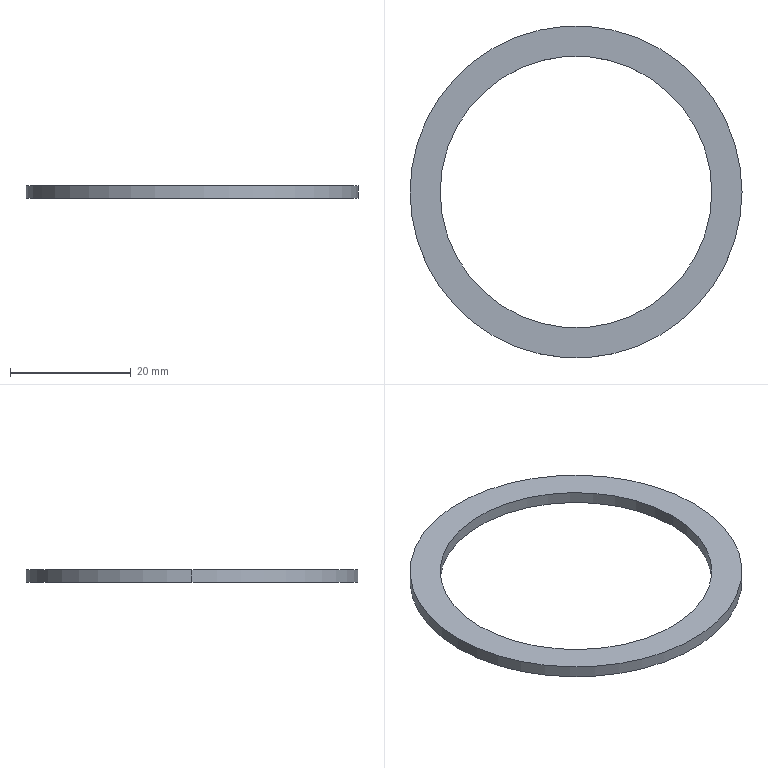Part | SolidWorks | features Extrusion 1 | 1 solid | 6 faces | box 55 x 55 x 2 mm | volume 1571 mm3 | cylinder 4 | plane 2 | commonest cylinder face diameters 45 x2 55 x2
STEP:
#1=CARTESIAN_POINT('',(-22.5,0.,2.));
#2=VERTEX_POINT('',#1);
#3=CARTESIAN_POINT('',(22.5,0.,2.));
#4=VERTEX_POINT('',#3);
#5=CARTESIAN_POINT('',(0.,0.,2.));
#6=DIRECTION('',(0.,0.,1.));
#7=DIRECTION('',(1.,0.,0.));
#8=AXIS2_PLACEMENT_3D('',#5,#6,#7);
#9=CIRCLE('',#8,22.5);
#10=EDGE_CURVE('',#2,#4,#9,.T.);
#11=ORIENTED_EDGE('',*,*,#10,.T.);
#12=CARTESIAN_POINT('',(22.5,0.,0.));
#13=VERTEX_POINT('',#12);
#14=CARTESIAN_POINT('',(22.5,0.,2.));
#15=DIRECTION('',(0.,0.,-1.));
#16=VECTOR('',#15,1000.);
#17=LINE('',#14,#16);
#18=EDGE_CURVE('',#4,#13,#17,.T.);
#19=ORIENTED_EDGE('',*,*,#18,.T.);
#20=CARTESIAN_POINT('',(-22.5,0.,0.));
#21=VERTEX_POINT('',#20);
#22=CARTESIAN_POINT('',(0.,0.,0.));
#23=DIRECTION('',(0.,0.,1.));
#24=DIRECTION('',(1.,0.,0.));
#25=AXIS2_PLACEMENT_3D('',#22,#23,#24);
#26=CIRCLE('',#25,22.5);
#27=EDGE_CURVE('',#21,#13,#26,.T.);
#28=ORIENTED_EDGE('',*,*,#27,.F.);
#29=CARTESIAN_POINT('',(-22.5,0.,2.));
#30=DIRECTION('',(0.,0.,-1.));
#31=VECTOR('',#30,1000.);
#32=LINE('',#29,#31);
#33=EDGE_CURVE('',#2,#21,#32,.T.);
#34=ORIENTED_EDGE('',*,*,#33,.F.);
#35=EDGE_LOOP('',(#11,#19,#28,#34));
#36=FACE_OUTER_BOUND('',#35,.T.);
#37=CARTESIAN_POINT('',(0.,0.,2.));
#38=DIRECTION('',(0.,0.,-1.));
#39=DIRECTION('',(-1.,0.,0.));
#40=AXIS2_PLACEMENT_3D('',#37,#38,#39);
#41=CYLINDRICAL_SURFACE('',#40,22.5);
#42=ADVANCED_FACE('',(#36),#41,.F.);
#43=CARTESIAN_POINT('',(27.5,0.,2.));
#44=VERTEX_POINT('',#43);
#45=CARTESIAN_POINT('',(-27.5,0.,2.));
#46=VERTEX_POINT('',#45);
#47=CARTESIAN_POINT('',(0.,0.,2.));
#48=DIRECTION('',(0.,0.,1.));
#49=DIRECTION('',(1.,0.,0.));
#50=AXIS2_PLACEMENT_3D('',#47,#48,#49);
#51=CIRCLE('',#50,27.5);
#52=EDGE_CURVE('',#44,#46,#51,.T.);
#53=ORIENTED_EDGE('',*,*,#52,.F.);
#54=CARTESIAN_POINT('',(27.5,0.,0.));
#55=VERTEX_POINT('',#54);
#56=CARTESIAN_POINT('',(27.5,0.,2.));
#57=DIRECTION('',(0.,0.,-1.));
#58=VECTOR('',#57,1000.);
#59=LINE('',#56,#58);
#60=EDGE_CURVE('',#44,#55,#59,.T.);
#61=ORIENTED_EDGE('',*,*,#60,.T.);
#62=CARTESIAN_POINT('',(-27.5,0.,0.));
#63=VERTEX_POINT('',#62);
#64=CARTESIAN_POINT('',(0.,0.,0.));
#65=DIRECTION('',(0.,0.,1.));
#66=DIRECTION('',(1.,0.,0.));
#67=AXIS2_PLACEMENT_3D('',#64,#65,#66);
#68=CIRCLE('',#67,27.5);
#69=EDGE_CURVE('',#55,#63,#68,.T.);
#70=ORIENTED_EDGE('',*,*,#69,.T.);
#71=CARTESIAN_POINT('',(-27.5,0.,2.));
#72=DIRECTION('',(0.,0.,-1.));
#73=VECTOR('',#72,1000.);
#74=LINE('',#71,#73);
#75=EDGE_CURVE('',#46,#63,#74,.T.);
#76=ORIENTED_EDGE('',*,*,#75,.F.);
#77=EDGE_LOOP('',(#53,#61,#70,#76));
#78=FACE_OUTER_BOUND('',#77,.T.);
#79=CARTESIAN_POINT('',(0.,0.,2.));
#80=DIRECTION('',(0.,0.,-1.));
#81=DIRECTION('',(-1.,0.,0.));
#82=AXIS2_PLACEMENT_3D('',#79,#80,#81);
#83=CYLINDRICAL_SURFACE('',#82,27.5);
#84=ADVANCED_FACE('',(#78),#83,.T.);
#85=CARTESIAN_POINT('',(0.,0.,2.));
#86=DIRECTION('',(0.,0.,1.));
#87=DIRECTION('',(1.,0.,0.));
#88=AXIS2_PLACEMENT_3D('',#85,#86,#87);
#89=CIRCLE('',#88,27.5);
#90=EDGE_CURVE('',#46,#44,#89,.T.);
#91=ORIENTED_EDGE('',*,*,#90,.T.);
#92=ORIENTED_EDGE('',*,*,#52,.T.);
#93=EDGE_LOOP('',(#91,#92));
#94=FACE_OUTER_BOUND('',#93,.T.);
#95=ORIENTED_EDGE('',*,*,#10,.F.);
#96=CARTESIAN_POINT('',(0.,0.,2.));
#97=DIRECTION('',(0.,0.,1.));
#98=DIRECTION('',(1.,0.,0.));
#99=AXIS2_PLACEMENT_3D('',#96,#97,#98);
#100=CIRCLE('',#99,22.5);
#101=EDGE_CURVE('',#4,#2,#100,.T.);
#102=ORIENTED_EDGE('',*,*,#101,.F.);
#103=EDGE_LOOP('',(#95,#102));
#104=FACE_BOUND('',#103,.T.);
#105=CARTESIAN_POINT('',(0.,0.,2.));
#106=DIRECTION('',(0.,0.,1.));
#107=DIRECTION('',(1.,0.,0.));
#108=AXIS2_PLACEMENT_3D('',#105,#106,#107);
#109=PLANE('',#108);
#110=ADVANCED_FACE('',(#94,#104),#109,.T.);
#111=CARTESIAN_POINT('',(0.,0.,0.));
#112=DIRECTION('',(0.,0.,1.));
#113=DIRECTION('',(1.,0.,0.));
#114=AXIS2_PLACEMENT_3D('',#111,#112,#113);
#115=CIRCLE('',#114,27.5);
#116=EDGE_CURVE('',#63,#55,#115,.T.);
#117=ORIENTED_EDGE('',*,*,#116,.F.);
#118=ORIENTED_EDGE('',*,*,#69,.F.);
#119=EDGE_LOOP('',(#117,#118));
#120=FACE_OUTER_BOUND('',#119,.T.);
#121=ORIENTED_EDGE('',*,*,#27,.T.);
#122=CARTESIAN_POINT('',(0.,0.,0.));
#123=DIRECTION('',(0.,0.,1.));
#124=DIRECTION('',(1.,0.,0.));
#125=AXIS2_PLACEMENT_3D('',#122,#123,#124);
#126=CIRCLE('',#125,22.5);
#127=EDGE_CURVE('',#13,#21,#126,.T.);
#128=ORIENTED_EDGE('',*,*,#127,.T.);
#129=EDGE_LOOP('',(#121,#128));
#130=FACE_BOUND('',#129,.T.);
#131=CARTESIAN_POINT('',(0.,0.,0.));
#132=DIRECTION('',(0.,0.,1.));
#133=DIRECTION('',(1.,0.,0.));
#134=AXIS2_PLACEMENT_3D('',#131,#132,#133);
#135=PLANE('',#134);
#136=ADVANCED_FACE('',(#120,#130),#135,.F.);
#137=ORIENTED_EDGE('',*,*,#60,.F.);
#138=ORIENTED_EDGE('',*,*,#90,.F.);
#139=ORIENTED_EDGE('',*,*,#75,.T.);
#140=ORIENTED_EDGE('',*,*,#116,.T.);
#141=EDGE_LOOP('',(#137,#138,#139,#140));
#142=FACE_OUTER_BOUND('',#141,.T.);
#143=CARTESIAN_POINT('',(0.,0.,2.));
#144=DIRECTION('',(0.,0.,-1.));
#145=DIRECTION('',(-1.,0.,0.));
#146=AXIS2_PLACEMENT_3D('',#143,#144,#145);
#147=CYLINDRICAL_SURFACE('',#146,27.5);
#148=ADVANCED_FACE('',(#142),#147,.T.);
#149=ORIENTED_EDGE('',*,*,#18,.F.);
#150=ORIENTED_EDGE('',*,*,#101,.T.);
#151=ORIENTED_EDGE('',*,*,#33,.T.);
#152=ORIENTED_EDGE('',*,*,#127,.F.);
#153=EDGE_LOOP('',(#149,#150,#151,#152));
#154=FACE_OUTER_BOUND('',#153,.T.);
#155=CARTESIAN_POINT('',(0.,0.,2.));
#156=DIRECTION('',(0.,0.,-1.));
#157=DIRECTION('',(-1.,0.,0.));
#158=AXIS2_PLACEMENT_3D('',#155,#156,#157);
#159=CYLINDRICAL_SURFACE('',#158,22.5);
#160=ADVANCED_FACE('',(#154),#159,.F.);
#161=CLOSED_SHELL('',(#42,#84,#110,#136,#148,#160));
#162=MANIFOLD_SOLID_BREP('',#161);
#163=CARTESIAN_POINT('',(0.,0.,0.));
#164=DIRECTION('',(0.,0.,1.));
#165=DIRECTION('',(1.,0.,0.));
#166=AXIS2_PLACEMENT_3D('',#163,#164,#165);
#167=(LENGTH_UNIT()NAMED_UNIT(*)SI_UNIT(.MILLI.,.METRE.));
#168=UNCERTAINTY_MEASURE_WITH_UNIT(LENGTH_MEASURE(0.00001),#167,'','');
#169=(NAMED_UNIT(*)PLANE_ANGLE_UNIT()SI_UNIT($,.RADIAN.));
#170=(NAMED_UNIT(*)SI_UNIT($,.STERADIAN.)SOLID_ANGLE_UNIT());
#171=(GEOMETRIC_REPRESENTATION_CONTEXT(3)GLOBAL_UNCERTAINTY_ASSIGNED_CONTEXT((#168))GLOBAL_UNIT_ASSIGNED_CONTEXT((#167,#169,#170))REPRESENTATION_CONTEXT('',''));
#172=ADVANCED_BREP_SHAPE_REPRESENTATION('',(#162,#166),#171);